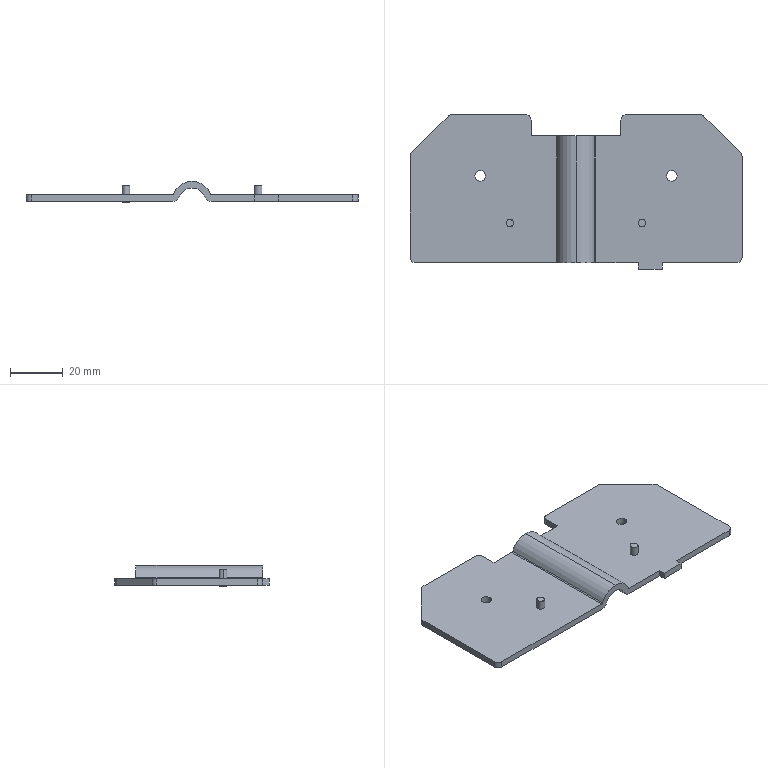Part | NX | features BREP 3 | 1 solid | 48 faces | box 125.7 x 58.5 x 8 mm | volume 16937 mm3 | cylinder 28 | plane 20 | commonest cylinder face diameters 4 x12 2.7 x4 3 x4 1 x2 6 x2 10 x2